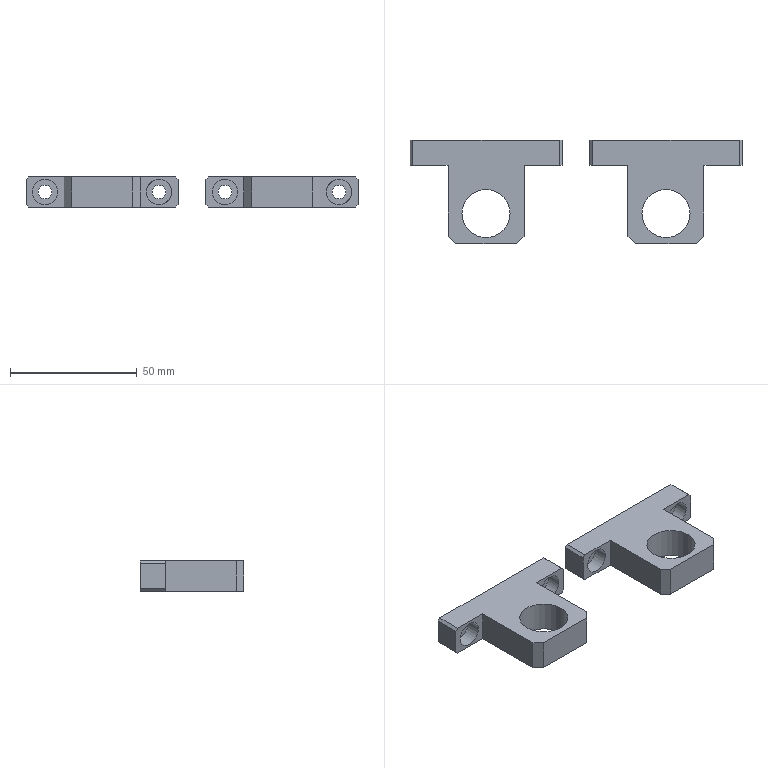CAM job | NX | 3-axis milling, drilling | part box 131 x 41 x 12 mm | stock box 136 x 46 x 15 mm
Tools:
number,name,description,diameter,corner_radius,flute_length,length,flutes
9,D10,平底铣刀-粗,10.0,0.0,35.0,75.0,2
12,D2-J,平底铣刀-精,2.0,0.0,50.0,75.0,2
7,D6-J,平底铣刀-精,6.0,0.0,25.0,75.0,2
10,D10-J,平底铣刀-精,10.0,0.0,35.0,75.0,2
1,D80R0.8飞刀,圆鼻刀-粗,80.0,0.8,50.0,75.0,2
1,D80R0.8飞刀-J,圆鼻刀-精,80.0,0.8,50.0,75.0,2
2,D6倒角刀,倒角刀,6.0,0.0,3.0,25.0,2
Operations:
program,operation,operation_type,tool,method,geometry_group,spindle_rpm,surface_speed,feed_per_tooth,feed_cut,feed_plunge,cut_length_mm,path_length_mm,cut_time_min,machine_time_min
B,底壁铣飞面一刀开粗_COPY,VolumeBased25DMillingOperation,D80R0.8飞刀,分层开粗-切深K-步距G,W-B,2800.0,703.696,0.5357,3000.0,100.0,1195.97,2325.948,0.3987,0.5117
B,底壁铣飞面一刀精光_COPY,VolumeBased25DMillingOperation,D80R0.8飞刀-J,侧刃精光-切深K-步距G,W-B,4000.0,1005.28,0.125,1000.0,100.0,238.998,334.998,0.239,0.2486
B,平面去毛刺6X45L_COPY,SurfaceContour,D6倒角刀,爬面_倒角-切深0-步距G,W-B,6500.0,122.519,0.1154,1500.0,100.0,478.618,878.017,0.3191,0.359
B,底壁铣倒角_COPY_1,VolumeBased25DMillingOperation,D6倒角刀,爬面_倒角-切深0-步距G,W-B,6500.0,122.519,0.1154,1500.0,100.0,75.202,508.818,0.0501,0.0935
A,顶面,FaceMilling,D80R0.8飞刀,侧刃精光-切深K-步距G,W-A,4500.0,1385.0,0.1667,1500.0,100.0,225.0,321.0,0.15,0.1596
A,动态开粗D10_COPY,CavityMilling,D10,动态开粗-切深K-步距K,W-A,8000.0,251.32,0.25,4000.0,100.0,5746.086,6690.014,1.437,1.531
A,底壁铣螺旋开粗-中_COPY,VolumeBased25DMillingOperation,D10,分层开粗-切深K-步距G,W-A,8000.0,251.327,0.125,2000.0,100.0,1886.561,2182.457,0.9433,0.9729
A,等高往复层切开粗-中_COPY,ZLevelMilling,D10,分层开粗-切深K-步距G,W-A,8000.0,251.32,0.25,4000.0,100.0,550.96,675.059,0.1377,0.1501
A,等高光顺清角D2参考6_COPY,ZLevelMilling,D2-J,分层精光-切深K-步距G,W-A,8000.0,50.266,0.0938,1500.0,100.0,3237.169,3832.122,2.158,2.218
A,打点-深0.8,Operation,D6倒角刀,NONE,W-A,8000.0,150.796,0.0312,500.0,90.0,3.6,179.207,0.0072,0.0248
A,仅选体,SurfaceContour,D6倒角刀,METHOD,W-A,8000.0,150.796,0.1875,3000.0,100.0,507.416,1270.282,0.1691,0.2454
A,铣倒角_1,PlanarMilling,D6倒角刀,METHOD,W-A,8000.0,150.796,0.0625,1000.0,100.0,125.15,400.404,0.1252,0.1527
A,底壁铣倒角_COPY,VolumeBased25DMillingOperation,D6倒角刀,爬面_倒角-切深0-步距G,W-A,6500.0,122.519,0.1154,1500.0,100.0,75.202,508.818,0.0501,0.0935
A,底壁铣螺旋精光-中_COPY,VolumeBased25DMillingOperation,D10-J,螺旋精光-切深K-步距G,W-A,8000.0,251.327,0.0375,600.0,100.0,251.039,548.567,0.4184,0.4482
A,外形半精_2,VolumeBased25DMillingOperation,D6-J,METHOD,W-A,9000.0,169.646,0.0667,1200.0,100.0,439.352,753.835,0.3661,0.3976